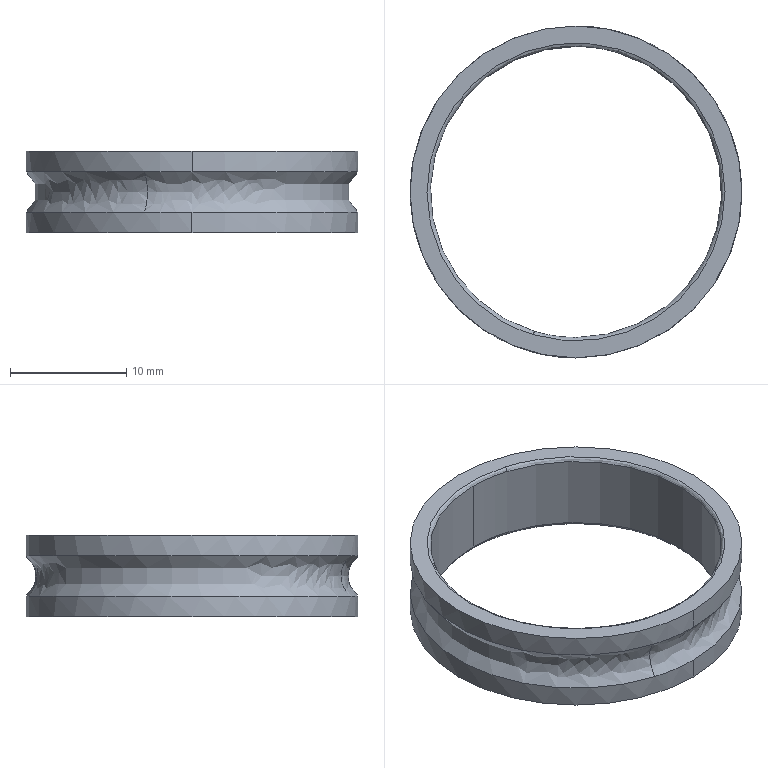Part | SolidWorks | features BaseBody 1 | 1 solid | 14 faces | box 28.5 x 28.5 x 7 mm | volume 836.369 mm3 | spline 6 | cylinder 6 | plane 2 | commonest cylinder face diameters 28.5 x4 25 x2
STEP:
#1=CARTESIAN_POINT('',(513.262,2.017,252.244));
#2=VERTEX_POINT('',#1);
#3=CARTESIAN_POINT('',(516.849,1.491,252.244));
#4=VERTEX_POINT('',#3);
#5=CARTESIAN_POINT('',(513.262,-10.483,252.244));
#6=DIRECTION('',(-0.000000004,0.00000001,-1.));
#7=DIRECTION('',(0.,-1.,-0.00000001));
#8=AXIS2_PLACEMENT_3D('',#5,#6,#7);
#9=CIRCLE('',#8,12.5);
#10=EDGE_CURVE('',#2,#4,#9,.T.);
#11=ORIENTED_EDGE('',*,*,#10,.T.);
#12=CARTESIAN_POINT('',(516.935,1.778,252.544));
#13=VERTEX_POINT('',#12);
#14=CARTESIAN_POINT('',(516.935,1.778,252.244));
#15=DIRECTION('',(-0.9579,0.287,0.000000007));
#16=DIRECTION('',(0.287,0.9579,0.000000008));
#17=AXIS2_PLACEMENT_3D('',#14,#15,#16);
#18=CIRCLE('',#17,0.3);
#19=EDGE_CURVE('',#4,#13,#18,.T.);
#20=ORIENTED_EDGE('',*,*,#19,.T.);
#21=CARTESIAN_POINT('',(509.588,-22.745,252.544));
#22=VERTEX_POINT('',#21);
#23=CARTESIAN_POINT('',(516.935,1.778,252.544));
#24=CARTESIAN_POINT('',(492.413,9.126,252.544));
#25=CARTESIAN_POINT('',(485.065,-15.397,252.544));
#26=CARTESIAN_POINT('',(509.588,-22.745,252.544));
#27=(BOUNDED_CURVE()B_SPLINE_CURVE(3,(#23,#24,#25,#26),.UNSPECIFIED.,.F.,.T.)B_SPLINE_CURVE_WITH_KNOTS((4,4),(0.,1.),.UNSPECIFIED.)CURVE()GEOMETRIC_REPRESENTATION_ITEM()RATIONAL_B_SPLINE_CURVE((1.,0.3333,0.3333,1.))REPRESENTATION_ITEM(''));
#28=EDGE_CURVE('',#13,#22,#27,.T.);
#29=ORIENTED_EDGE('',*,*,#28,.T.);
#30=CARTESIAN_POINT('',(509.674,-22.457,252.244));
#31=VERTEX_POINT('',#30);
#32=CARTESIAN_POINT('',(509.588,-22.745,252.244));
#33=DIRECTION('',(0.9579,-0.287,-0.000000007));
#34=DIRECTION('',(-0.287,-0.9579,-0.000000008));
#35=AXIS2_PLACEMENT_3D('',#32,#33,#34);
#36=CIRCLE('',#35,0.3);
#37=EDGE_CURVE('',#31,#22,#36,.T.);
#38=ORIENTED_EDGE('',*,*,#37,.F.);
#39=CARTESIAN_POINT('',(513.262,-10.483,252.244));
#40=DIRECTION('',(-0.000000004,0.00000001,-1.));
#41=DIRECTION('',(0.,-1.,-0.00000001));
#42=AXIS2_PLACEMENT_3D('',#39,#40,#41);
#43=CIRCLE('',#42,12.5);
#44=EDGE_CURVE('',#31,#2,#43,.T.);
#45=ORIENTED_EDGE('',*,*,#44,.T.);
#46=EDGE_LOOP('',(#11,#20,#29,#38,#45));
#47=FACE_OUTER_BOUND('',#46,.T.);
#48=CARTESIAN_POINT('',(516.849,1.491,252.244));
#49=CARTESIAN_POINT('',(492.901,8.666,252.244));
#50=CARTESIAN_POINT('',(485.726,-15.282,252.244));
#51=CARTESIAN_POINT('',(509.674,-22.457,252.244));
#52=CARTESIAN_POINT('',(516.849,1.491,252.42));
#53=CARTESIAN_POINT('',(492.901,8.666,252.42));
#54=CARTESIAN_POINT('',(485.726,-15.282,252.42));
#55=CARTESIAN_POINT('',(509.674,-22.457,252.42));
#56=CARTESIAN_POINT('',(516.885,1.61,252.544));
#57=CARTESIAN_POINT('',(492.699,8.857,252.544));
#58=CARTESIAN_POINT('',(485.452,-15.33,252.544));
#59=CARTESIAN_POINT('',(509.638,-22.576,252.544));
#60=CARTESIAN_POINT('',(516.935,1.778,252.544));
#61=CARTESIAN_POINT('',(492.413,9.126,252.544));
#62=CARTESIAN_POINT('',(485.065,-15.397,252.544));
#63=CARTESIAN_POINT('',(509.588,-22.745,252.544));
#64=(BOUNDED_SURFACE()B_SPLINE_SURFACE(3,3,((#48,#49,#50,#51),(#52,#53,#54,#55),(#56,#57,#58,#59),(#60,#61,#62,#63)),.UNSPECIFIED.,.F.,.F.,.T.)B_SPLINE_SURFACE_WITH_KNOTS((4,4),(4,4),(0.,1.),(0.,1.),.UNSPECIFIED.)GEOMETRIC_REPRESENTATION_ITEM()RATIONAL_B_SPLINE_SURFACE(((1.,0.3333,0.3333,1.),(0.8047,0.2682,0.2682,0.8047),(0.8047,0.2682,0.2682,0.8047),(1.,0.3333,0.3333,1.)))REPRESENTATION_ITEM('')SURFACE());
#65=ADVANCED_FACE('',(#47),#64,.T.);
#66=CARTESIAN_POINT('',(509.588,-22.745,245.544));
#67=VERTEX_POINT('',#66);
#68=CARTESIAN_POINT('',(516.935,1.778,245.544));
#69=VERTEX_POINT('',#68);
#70=CARTESIAN_POINT('',(509.588,-22.745,245.544));
#71=CARTESIAN_POINT('',(485.065,-15.397,245.544));
#72=CARTESIAN_POINT('',(492.413,9.126,245.544));
#73=CARTESIAN_POINT('',(516.935,1.778,245.544));
#74=(BOUNDED_CURVE()B_SPLINE_CURVE(3,(#70,#71,#72,#73),.UNSPECIFIED.,.F.,.T.)B_SPLINE_CURVE_WITH_KNOTS((4,4),(0.,1.),.UNSPECIFIED.)CURVE()GEOMETRIC_REPRESENTATION_ITEM()RATIONAL_B_SPLINE_CURVE((1.,0.3333,0.3333,1.))REPRESENTATION_ITEM(''));
#75=EDGE_CURVE('',#67,#69,#74,.T.);
#76=ORIENTED_EDGE('',*,*,#75,.T.);
#77=CARTESIAN_POINT('',(516.849,1.491,245.844));
#78=VERTEX_POINT('',#77);
#79=CARTESIAN_POINT('',(516.935,1.778,245.844));
#80=DIRECTION('',(-0.9579,0.287,0.000000007));
#81=DIRECTION('',(0.287,0.9579,0.000000008));
#82=AXIS2_PLACEMENT_3D('',#79,#80,#81);
#83=CIRCLE('',#82,0.3);
#84=EDGE_CURVE('',#69,#78,#83,.T.);
#85=ORIENTED_EDGE('',*,*,#84,.T.);
#86=CARTESIAN_POINT('',(513.262,2.017,245.844));
#87=VERTEX_POINT('',#86);
#88=CARTESIAN_POINT('',(513.262,-10.483,245.844));
#89=DIRECTION('',(0.000000004,-0.00000001,1.));
#90=DIRECTION('',(0.,-1.,-0.00000001));
#91=AXIS2_PLACEMENT_3D('',#88,#89,#90);
#92=CIRCLE('',#91,12.5);
#93=EDGE_CURVE('',#78,#87,#92,.T.);
#94=ORIENTED_EDGE('',*,*,#93,.T.);
#95=CARTESIAN_POINT('',(509.674,-22.457,245.844));
#96=VERTEX_POINT('',#95);
#97=CARTESIAN_POINT('',(513.262,-10.483,245.844));
#98=DIRECTION('',(0.000000004,-0.00000001,1.));
#99=DIRECTION('',(0.,-1.,-0.00000001));
#100=AXIS2_PLACEMENT_3D('',#97,#98,#99);
#101=CIRCLE('',#100,12.5);
#102=EDGE_CURVE('',#87,#96,#101,.T.);
#103=ORIENTED_EDGE('',*,*,#102,.T.);
#104=CARTESIAN_POINT('',(509.588,-22.745,245.844));
#105=DIRECTION('',(0.9579,-0.287,-0.000000007));
#106=DIRECTION('',(-0.287,-0.9579,-0.000000008));
#107=AXIS2_PLACEMENT_3D('',#104,#105,#106);
#108=CIRCLE('',#107,0.3);
#109=EDGE_CURVE('',#67,#96,#108,.T.);
#110=ORIENTED_EDGE('',*,*,#109,.F.);
#111=EDGE_LOOP('',(#76,#85,#94,#103,#110));
#112=FACE_OUTER_BOUND('',#111,.T.);
#113=CARTESIAN_POINT('',(516.935,1.778,245.544));
#114=CARTESIAN_POINT('',(492.413,9.126,245.544));
#115=CARTESIAN_POINT('',(485.065,-15.397,245.544));
#116=CARTESIAN_POINT('',(509.588,-22.745,245.544));
#117=CARTESIAN_POINT('',(516.885,1.61,245.544));
#118=CARTESIAN_POINT('',(492.699,8.857,245.544));
#119=CARTESIAN_POINT('',(485.452,-15.33,245.544));
#120=CARTESIAN_POINT('',(509.638,-22.576,245.544));
#121=CARTESIAN_POINT('',(516.849,1.491,245.669));
#122=CARTESIAN_POINT('',(492.901,8.666,245.669));
#123=CARTESIAN_POINT('',(485.726,-15.282,245.669));
#124=CARTESIAN_POINT('',(509.674,-22.457,245.669));
#125=CARTESIAN_POINT('',(516.849,1.491,245.844));
#126=CARTESIAN_POINT('',(492.901,8.666,245.844));
#127=CARTESIAN_POINT('',(485.726,-15.282,245.844));
#128=CARTESIAN_POINT('',(509.674,-22.457,245.844));
#129=(BOUNDED_SURFACE()B_SPLINE_SURFACE(3,3,((#113,#114,#115,#116),(#117,#118,#119,#120),(#121,#122,#123,#124),(#125,#126,#127,#128)),.UNSPECIFIED.,.F.,.F.,.T.)B_SPLINE_SURFACE_WITH_KNOTS((4,4),(4,4),(0.,1.),(0.,1.),.UNSPECIFIED.)GEOMETRIC_REPRESENTATION_ITEM()RATIONAL_B_SPLINE_SURFACE(((1.,0.3333,0.3333,1.),(0.8047,0.2682,0.2682,0.8047),(0.8047,0.2682,0.2682,0.8047),(1.,0.3333,0.3333,1.)))REPRESENTATION_ITEM('')SURFACE());
#130=ADVANCED_FACE('',(#112),#129,.T.);
#131=CARTESIAN_POINT('',(517.352,3.167,247.321));
#132=VERTEX_POINT('',#131);
#133=CARTESIAN_POINT('',(513.262,-24.733,247.321));
#134=VERTEX_POINT('',#133);
#135=CARTESIAN_POINT('',(513.262,-10.483,247.321));
#136=DIRECTION('',(-0.000000004,0.00000001,-1.));
#137=DIRECTION('',(0.,-1.,-0.00000001));
#138=AXIS2_PLACEMENT_3D('',#135,#136,#137);
#139=CIRCLE('',#138,14.25);
#140=EDGE_CURVE('',#132,#134,#139,.T.);
#141=ORIENTED_EDGE('',*,*,#140,.F.);
#142=CARTESIAN_POINT('',(517.352,3.167,250.768));
#143=VERTEX_POINT('',#142);
#144=CARTESIAN_POINT('',(517.696,4.317,249.044));
#145=DIRECTION('',(-0.9579,0.287,0.000000007));
#146=DIRECTION('',(0.287,0.9579,0.000000008));
#147=AXIS2_PLACEMENT_3D('',#144,#145,#146);
#148=CIRCLE('',#147,2.1);
#149=EDGE_CURVE('',#132,#143,#148,.T.);
#150=ORIENTED_EDGE('',*,*,#149,.T.);
#151=CARTESIAN_POINT('',(513.262,-24.733,250.768));
#152=VERTEX_POINT('',#151);
#153=CARTESIAN_POINT('',(513.262,-10.483,250.768));
#154=DIRECTION('',(0.000000004,-0.00000001,1.));
#155=DIRECTION('',(0.,-1.,-0.00000001));
#156=AXIS2_PLACEMENT_3D('',#153,#154,#155);
#157=CIRCLE('',#156,14.25);
#158=EDGE_CURVE('',#152,#143,#157,.T.);
#159=ORIENTED_EDGE('',*,*,#158,.F.);
#160=CARTESIAN_POINT('',(509.171,-24.134,250.768));
#161=VERTEX_POINT('',#160);
#162=CARTESIAN_POINT('',(513.262,-10.483,250.768));
#163=DIRECTION('',(0.000000004,-0.00000001,1.));
#164=DIRECTION('',(0.,-1.,-0.00000001));
#165=AXIS2_PLACEMENT_3D('',#162,#163,#164);
#166=CIRCLE('',#165,14.25);
#167=EDGE_CURVE('',#161,#152,#166,.T.);
#168=ORIENTED_EDGE('',*,*,#167,.F.);
#169=CARTESIAN_POINT('',(509.171,-24.134,247.321));
#170=VERTEX_POINT('',#169);
#171=CARTESIAN_POINT('',(508.827,-25.283,249.044));
#172=DIRECTION('',(0.9579,-0.287,-0.000000007));
#173=DIRECTION('',(-0.287,-0.9579,-0.000000008));
#174=AXIS2_PLACEMENT_3D('',#171,#172,#173);
#175=CIRCLE('',#174,2.1);
#176=EDGE_CURVE('',#170,#161,#175,.T.);
#177=ORIENTED_EDGE('',*,*,#176,.F.);
#178=CARTESIAN_POINT('',(513.262,-10.483,247.321));
#179=DIRECTION('',(-0.000000004,0.00000001,-1.));
#180=DIRECTION('',(0.,-1.,-0.00000001));
#181=AXIS2_PLACEMENT_3D('',#178,#179,#180);
#182=CIRCLE('',#181,14.25);
#183=EDGE_CURVE('',#134,#170,#182,.T.);
#184=ORIENTED_EDGE('',*,*,#183,.F.);
#185=EDGE_LOOP('',(#141,#150,#159,#168,#177,#184));
#186=FACE_OUTER_BOUND('',#185,.T.);
#187=CARTESIAN_POINT('',(509.171,-24.134,247.321));
#188=CARTESIAN_POINT('',(536.472,-32.314,247.321));
#189=CARTESIAN_POINT('',(544.652,-5.013,247.321));
#190=CARTESIAN_POINT('',(517.352,3.167,247.321));
#191=CARTESIAN_POINT('',(509.55,-22.869,248.24));
#192=CARTESIAN_POINT('',(534.322,-30.292,248.24));
#193=CARTESIAN_POINT('',(541.745,-5.52,248.24));
#194=CARTESIAN_POINT('',(516.973,1.903,248.24));
#195=CARTESIAN_POINT('',(509.55,-22.869,249.848));
#196=CARTESIAN_POINT('',(534.322,-30.292,249.848));
#197=CARTESIAN_POINT('',(541.745,-5.52,249.848));
#198=CARTESIAN_POINT('',(516.973,1.903,249.848));
#199=CARTESIAN_POINT('',(509.171,-24.134,250.768));
#200=CARTESIAN_POINT('',(536.472,-32.314,250.768));
#201=CARTESIAN_POINT('',(544.652,-5.013,250.768));
#202=CARTESIAN_POINT('',(517.352,3.167,250.768));
#203=(BOUNDED_SURFACE()B_SPLINE_SURFACE(3,3,((#187,#188,#189,#190),(#191,#192,#193,#194),(#195,#196,#197,#198),(#199,#200,#201,#202)),.UNSPECIFIED.,.F.,.F.,.T.)B_SPLINE_SURFACE_WITH_KNOTS((4,4),(4,4),(0.,1.),(0.,1.),.UNSPECIFIED.)GEOMETRIC_REPRESENTATION_ITEM()RATIONAL_B_SPLINE_SURFACE(((1.,0.3333,0.3333,1.),(0.7143,0.2381,0.2381,0.7143),(0.7143,0.2381,0.2381,0.7143),(1.,0.3333,0.3333,1.)))REPRESENTATION_ITEM('')SURFACE());
#204=ADVANCED_FACE('',(#186),#203,.F.);
#205=ORIENTED_EDGE('',*,*,#102,.F.);
#206=CARTESIAN_POINT('',(513.262,2.017,249.044));
#207=DIRECTION('',(0.000000004,-0.00000001,1.));
#208=VECTOR('',#207,1000.);
#209=LINE('',#206,#208);
#210=EDGE_CURVE('',#87,#2,#209,.T.);
#211=ORIENTED_EDGE('',*,*,#210,.T.);
#212=ORIENTED_EDGE('',*,*,#44,.F.);
#213=CARTESIAN_POINT('',(513.262,-22.983,252.244));
#214=VERTEX_POINT('',#213);
#215=CARTESIAN_POINT('',(513.262,-10.483,252.244));
#216=DIRECTION('',(-0.000000004,0.00000001,-1.));
#217=DIRECTION('',(0.,-1.,-0.00000001));
#218=AXIS2_PLACEMENT_3D('',#215,#216,#217);
#219=CIRCLE('',#218,12.5);
#220=EDGE_CURVE('',#214,#31,#219,.T.);
#221=ORIENTED_EDGE('',*,*,#220,.F.);
#222=CARTESIAN_POINT('',(513.262,-22.983,245.844));
#223=VERTEX_POINT('',#222);
#224=CARTESIAN_POINT('',(513.262,-22.983,249.044));
#225=DIRECTION('',(0.000000004,-0.00000001,1.));
#226=VECTOR('',#225,1000.);
#227=LINE('',#224,#226);
#228=EDGE_CURVE('',#223,#214,#227,.T.);
#229=ORIENTED_EDGE('',*,*,#228,.F.);
#230=CARTESIAN_POINT('',(513.262,-10.483,245.844));
#231=DIRECTION('',(0.000000004,-0.00000001,1.));
#232=DIRECTION('',(0.,-1.,-0.00000001));
#233=AXIS2_PLACEMENT_3D('',#230,#231,#232);
#234=CIRCLE('',#233,12.5);
#235=EDGE_CURVE('',#96,#223,#234,.T.);
#236=ORIENTED_EDGE('',*,*,#235,.F.);
#237=EDGE_LOOP('',(#205,#211,#212,#221,#229,#236));
#238=FACE_OUTER_BOUND('',#237,.T.);
#239=CARTESIAN_POINT('',(513.262,-10.483,249.044));
#240=DIRECTION('',(0.000000004,-0.00000001,1.));
#241=DIRECTION('',(0.,-1.,-0.00000001));
#242=AXIS2_PLACEMENT_3D('',#239,#240,#241);
#243=CYLINDRICAL_SURFACE('',#242,12.5);
#244=ADVANCED_FACE('',(#238),#243,.F.);
#245=ORIENTED_EDGE('',*,*,#158,.T.);
#246=CARTESIAN_POINT('',(513.262,3.767,250.768));
#247=VERTEX_POINT('',#246);
#248=CARTESIAN_POINT('',(513.262,-10.483,250.768));
#249=DIRECTION('',(0.000000004,-0.00000001,1.));
#250=DIRECTION('',(0.,-1.,-0.00000001));
#251=AXIS2_PLACEMENT_3D('',#248,#249,#250);
#252=CIRCLE('',#251,14.25);
#253=EDGE_CURVE('',#143,#247,#252,.T.);
#254=ORIENTED_EDGE('',*,*,#253,.T.);
#255=CARTESIAN_POINT('',(513.262,3.767,252.544));
#256=VERTEX_POINT('',#255);
#257=CARTESIAN_POINT('',(513.262,3.767,251.656));
#258=DIRECTION('',(0.000000004,-0.00000001,1.));
#259=VECTOR('',#258,1000.);
#260=LINE('',#257,#259);
#261=EDGE_CURVE('',#247,#256,#260,.T.);
#262=ORIENTED_EDGE('',*,*,#261,.T.);
#263=CARTESIAN_POINT('',(513.262,-24.733,252.544));
#264=VERTEX_POINT('',#263);
#265=CARTESIAN_POINT('',(513.262,-10.483,252.544));
#266=DIRECTION('',(0.000000004,-0.00000001,1.));
#267=DIRECTION('',(0.,-1.,-0.00000001));
#268=AXIS2_PLACEMENT_3D('',#265,#266,#267);
#269=CIRCLE('',#268,14.25);
#270=EDGE_CURVE('',#264,#256,#269,.T.);
#271=ORIENTED_EDGE('',*,*,#270,.F.);
#272=CARTESIAN_POINT('',(513.262,-24.733,251.656));
#273=DIRECTION('',(0.000000004,-0.00000001,1.));
#274=VECTOR('',#273,1000.);
#275=LINE('',#272,#274);
#276=EDGE_CURVE('',#152,#264,#275,.T.);
#277=ORIENTED_EDGE('',*,*,#276,.F.);
#278=EDGE_LOOP('',(#245,#254,#262,#271,#277));
#279=FACE_OUTER_BOUND('',#278,.T.);
#280=CARTESIAN_POINT('',(513.262,-10.483,251.656));
#281=DIRECTION('',(0.000000004,-0.00000001,1.));
#282=DIRECTION('',(0.,-1.,-0.00000001));
#283=AXIS2_PLACEMENT_3D('',#280,#281,#282);
#284=CYLINDRICAL_SURFACE('',#283,14.25);
#285=ADVANCED_FACE('',(#279),#284,.T.);
#286=CARTESIAN_POINT('',(513.262,3.767,245.544));
#287=VERTEX_POINT('',#286);
#288=CARTESIAN_POINT('',(513.262,-24.733,245.544));
#289=VERTEX_POINT('',#288);
#290=CARTESIAN_POINT('',(513.262,-10.483,245.544));
#291=DIRECTION('',(-0.000000004,0.00000001,-1.));
#292=DIRECTION('',(0.,-1.,-0.00000001));
#293=AXIS2_PLACEMENT_3D('',#290,#291,#292);
#294=CIRCLE('',#293,14.25);
#295=EDGE_CURVE('',#287,#289,#294,.T.);
#296=ORIENTED_EDGE('',*,*,#295,.F.);
#297=CARTESIAN_POINT('',(513.262,3.767,247.321));
#298=VERTEX_POINT('',#297);
#299=CARTESIAN_POINT('',(513.262,3.767,246.433));
#300=DIRECTION('',(0.000000004,-0.00000001,1.));
#301=VECTOR('',#300,1000.);
#302=LINE('',#299,#301);
#303=EDGE_CURVE('',#287,#298,#302,.T.);
#304=ORIENTED_EDGE('',*,*,#303,.T.);
#305=CARTESIAN_POINT('',(513.262,-10.483,247.321));
#306=DIRECTION('',(-0.000000004,0.00000001,-1.));
#307=DIRECTION('',(0.,-1.,-0.00000001));
#308=AXIS2_PLACEMENT_3D('',#305,#306,#307);
#309=CIRCLE('',#308,14.25);
#310=EDGE_CURVE('',#298,#132,#309,.T.);
#311=ORIENTED_EDGE('',*,*,#310,.T.);
#312=ORIENTED_EDGE('',*,*,#140,.T.);
#313=CARTESIAN_POINT('',(513.262,-24.733,246.433));
#314=DIRECTION('',(0.000000004,-0.00000001,1.));
#315=VECTOR('',#314,1000.);
#316=LINE('',#313,#315);
#317=EDGE_CURVE('',#289,#134,#316,.T.);
#318=ORIENTED_EDGE('',*,*,#317,.F.);
#319=EDGE_LOOP('',(#296,#304,#311,#312,#318));
#320=FACE_OUTER_BOUND('',#319,.T.);
#321=CARTESIAN_POINT('',(513.262,-10.483,246.433));
#322=DIRECTION('',(0.000000004,-0.00000001,1.));
#323=DIRECTION('',(0.,-1.,-0.00000001));
#324=AXIS2_PLACEMENT_3D('',#321,#322,#323);
#325=CYLINDRICAL_SURFACE('',#324,14.25);
#326=ADVANCED_FACE('',(#320),#325,.T.);
#327=ORIENTED_EDGE('',*,*,#210,.F.);
#328=ORIENTED_EDGE('',*,*,#93,.F.);
#329=CARTESIAN_POINT('',(513.262,-10.483,245.844));
#330=DIRECTION('',(0.000000004,-0.00000001,1.));
#331=DIRECTION('',(0.,-1.,-0.00000001));
#332=AXIS2_PLACEMENT_3D('',#329,#330,#331);
#333=CIRCLE('',#332,12.5);
#334=EDGE_CURVE('',#223,#78,#333,.T.);
#335=ORIENTED_EDGE('',*,*,#334,.F.);
#336=ORIENTED_EDGE('',*,*,#228,.T.);
#337=CARTESIAN_POINT('',(513.262,-10.483,252.244));
#338=DIRECTION('',(-0.000000004,0.00000001,-1.));
#339=DIRECTION('',(0.,-1.,-0.00000001));
#340=AXIS2_PLACEMENT_3D('',#337,#338,#339);
#341=CIRCLE('',#340,12.5);
#342=EDGE_CURVE('',#4,#214,#341,.T.);
#343=ORIENTED_EDGE('',*,*,#342,.F.);
#344=ORIENTED_EDGE('',*,*,#10,.F.);
#345=EDGE_LOOP('',(#327,#328,#335,#336,#343,#344));
#346=FACE_OUTER_BOUND('',#345,.T.);
#347=CARTESIAN_POINT('',(513.262,-10.483,249.044));
#348=DIRECTION('',(0.000000004,-0.00000001,1.));
#349=DIRECTION('',(0.,-1.,-0.00000001));
#350=AXIS2_PLACEMENT_3D('',#347,#348,#349);
#351=CYLINDRICAL_SURFACE('',#350,12.5);
#352=ADVANCED_FACE('',(#346),#351,.F.);
#353=ORIENTED_EDGE('',*,*,#19,.F.);
#354=ORIENTED_EDGE('',*,*,#342,.T.);
#355=ORIENTED_EDGE('',*,*,#220,.T.);
#356=ORIENTED_EDGE('',*,*,#37,.T.);
#357=CARTESIAN_POINT('',(509.588,-22.745,252.544));
#358=CARTESIAN_POINT('',(534.111,-30.093,252.544));
#359=CARTESIAN_POINT('',(541.458,-5.57,252.544));
#360=CARTESIAN_POINT('',(516.935,1.778,252.544));
#361=(BOUNDED_CURVE()B_SPLINE_CURVE(3,(#357,#358,#359,#360),.UNSPECIFIED.,.F.,.T.)B_SPLINE_CURVE_WITH_KNOTS((4,4),(0.,1.),.UNSPECIFIED.)CURVE()GEOMETRIC_REPRESENTATION_ITEM()RATIONAL_B_SPLINE_CURVE((1.,0.3333,0.3333,1.))REPRESENTATION_ITEM(''));
#362=EDGE_CURVE('',#22,#13,#361,.T.);
#363=ORIENTED_EDGE('',*,*,#362,.T.);
#364=EDGE_LOOP('',(#353,#354,#355,#356,#363));
#365=FACE_OUTER_BOUND('',#364,.T.);
#366=CARTESIAN_POINT('',(509.674,-22.457,252.244));
#367=CARTESIAN_POINT('',(533.622,-29.633,252.244));
#368=CARTESIAN_POINT('',(540.797,-5.685,252.244));
#369=CARTESIAN_POINT('',(516.849,1.491,252.244));
#370=CARTESIAN_POINT('',(509.674,-22.457,252.42));
#371=CARTESIAN_POINT('',(533.622,-29.633,252.42));
#372=CARTESIAN_POINT('',(540.797,-5.685,252.42));
#373=CARTESIAN_POINT('',(516.849,1.491,252.42));
#374=CARTESIAN_POINT('',(509.638,-22.576,252.544));
#375=CARTESIAN_POINT('',(533.824,-29.823,252.544));
#376=CARTESIAN_POINT('',(541.071,-5.637,252.544));
#377=CARTESIAN_POINT('',(516.885,1.61,252.544));
#378=CARTESIAN_POINT('',(509.588,-22.745,252.544));
#379=CARTESIAN_POINT('',(534.111,-30.093,252.544));
#380=CARTESIAN_POINT('',(541.458,-5.57,252.544));
#381=CARTESIAN_POINT('',(516.935,1.778,252.544));
#382=(BOUNDED_SURFACE()B_SPLINE_SURFACE(3,3,((#366,#367,#368,#369),(#370,#371,#372,#373),(#374,#375,#376,#377),(#378,#379,#380,#381)),.UNSPECIFIED.,.F.,.F.,.F.)B_SPLINE_SURFACE_WITH_KNOTS((4,4),(4,4),(0.,1.),(0.,1.),.UNSPECIFIED.)GEOMETRIC_REPRESENTATION_ITEM()RATIONAL_B_SPLINE_SURFACE(((1.,0.3333,0.3333,1.),(0.8047,0.2682,0.2682,0.8047),(0.8047,0.2682,0.2682,0.8047),(1.,0.3333,0.3333,1.)))REPRESENTATION_ITEM('')SURFACE());
#383=ADVANCED_FACE('',(#365),#382,.T.);
#384=ORIENTED_EDGE('',*,*,#84,.F.);
#385=CARTESIAN_POINT('',(516.935,1.778,245.544));
#386=CARTESIAN_POINT('',(541.458,-5.57,245.544));
#387=CARTESIAN_POINT('',(534.111,-30.093,245.544));
#388=CARTESIAN_POINT('',(509.588,-22.745,245.544));
#389=(BOUNDED_CURVE()B_SPLINE_CURVE(3,(#385,#386,#387,#388),.UNSPECIFIED.,.F.,.T.)B_SPLINE_CURVE_WITH_KNOTS((4,4),(0.,1.),.UNSPECIFIED.)CURVE()GEOMETRIC_REPRESENTATION_ITEM()RATIONAL_B_SPLINE_CURVE((1.,0.3333,0.3333,1.))REPRESENTATION_ITEM(''));
#390=EDGE_CURVE('',#69,#67,#389,.T.);
#391=ORIENTED_EDGE('',*,*,#390,.T.);
#392=ORIENTED_EDGE('',*,*,#109,.T.);
#393=ORIENTED_EDGE('',*,*,#235,.T.);
#394=ORIENTED_EDGE('',*,*,#334,.T.);
#395=EDGE_LOOP('',(#384,#391,#392,#393,#394));
#396=FACE_OUTER_BOUND('',#395,.T.);
#397=CARTESIAN_POINT('',(509.588,-22.745,245.544));
#398=CARTESIAN_POINT('',(534.111,-30.093,245.544));
#399=CARTESIAN_POINT('',(541.458,-5.57,245.544));
#400=CARTESIAN_POINT('',(516.935,1.778,245.544));
#401=CARTESIAN_POINT('',(509.638,-22.576,245.544));
#402=CARTESIAN_POINT('',(533.824,-29.823,245.544));
#403=CARTESIAN_POINT('',(541.071,-5.637,245.544));
#404=CARTESIAN_POINT('',(516.885,1.61,245.544));
#405=CARTESIAN_POINT('',(509.674,-22.457,245.669));
#406=CARTESIAN_POINT('',(533.622,-29.633,245.669));
#407=CARTESIAN_POINT('',(540.797,-5.685,245.669));
#408=CARTESIAN_POINT('',(516.849,1.491,245.669));
#409=CARTESIAN_POINT('',(509.674,-22.457,245.844));
#410=CARTESIAN_POINT('',(533.622,-29.633,245.844));
#411=CARTESIAN_POINT('',(540.797,-5.685,245.844));
#412=CARTESIAN_POINT('',(516.849,1.491,245.844));
#413=(BOUNDED_SURFACE()B_SPLINE_SURFACE(3,3,((#397,#398,#399,#400),(#401,#402,#403,#404),(#405,#406,#407,#408),(#409,#410,#411,#412)),.UNSPECIFIED.,.F.,.F.,.T.)B_SPLINE_SURFACE_WITH_KNOTS((4,4),(4,4),(0.,1.),(0.,1.),.UNSPECIFIED.)GEOMETRIC_REPRESENTATION_ITEM()RATIONAL_B_SPLINE_SURFACE(((1.,0.3333,0.3333,1.),(0.8047,0.2682,0.2682,0.8047),(0.8047,0.2682,0.2682,0.8047),(1.,0.3333,0.3333,1.)))REPRESENTATION_ITEM('')SURFACE());
#414=ADVANCED_FACE('',(#396),#413,.T.);
#415=ORIENTED_EDGE('',*,*,#28,.F.);
#416=ORIENTED_EDGE('',*,*,#362,.F.);
#417=EDGE_LOOP('',(#415,#416));
#418=FACE_BOUND('',#417,.T.);
#419=ORIENTED_EDGE('',*,*,#270,.T.);
#420=CARTESIAN_POINT('',(513.262,-10.483,252.544));
#421=DIRECTION('',(0.000000004,-0.00000001,1.));
#422=DIRECTION('',(0.,-1.,-0.00000001));
#423=AXIS2_PLACEMENT_3D('',#420,#421,#422);
#424=CIRCLE('',#423,14.25);
#425=EDGE_CURVE('',#256,#264,#424,.T.);
#426=ORIENTED_EDGE('',*,*,#425,.T.);
#427=EDGE_LOOP('',(#419,#426));
#428=FACE_OUTER_BOUND('',#427,.T.);
#429=CARTESIAN_POINT('',(509.38,-23.439,252.544));
#430=DIRECTION('',(0.000000004,-0.00000001,1.));
#431=DIRECTION('',(0.,-1.,-0.00000001));
#432=AXIS2_PLACEMENT_3D('',#429,#430,#431);
#433=PLANE('',#432);
#434=ADVANCED_FACE('',(#418,#428),#433,.T.);
#435=CARTESIAN_POINT('',(513.262,-10.483,245.544));
#436=DIRECTION('',(-0.000000004,0.00000001,-1.));
#437=DIRECTION('',(0.,-1.,-0.00000001));
#438=AXIS2_PLACEMENT_3D('',#435,#436,#437);
#439=CIRCLE('',#438,14.25);
#440=EDGE_CURVE('',#289,#287,#439,.T.);
#441=ORIENTED_EDGE('',*,*,#440,.T.);
#442=ORIENTED_EDGE('',*,*,#295,.T.);
#443=EDGE_LOOP('',(#441,#442));
#444=FACE_OUTER_BOUND('',#443,.T.);
#445=ORIENTED_EDGE('',*,*,#75,.F.);
#446=ORIENTED_EDGE('',*,*,#390,.F.);
#447=EDGE_LOOP('',(#445,#446));
#448=FACE_BOUND('',#447,.T.);
#449=CARTESIAN_POINT('',(509.38,-23.439,245.544));
#450=DIRECTION('',(-0.000000004,0.00000001,-1.));
#451=DIRECTION('',(0.,1.,0.00000001));
#452=AXIS2_PLACEMENT_3D('',#449,#450,#451);
#453=PLANE('',#452);
#454=ADVANCED_FACE('',(#444,#448),#453,.T.);
#455=ORIENTED_EDGE('',*,*,#261,.F.);
#456=CARTESIAN_POINT('',(513.262,-10.483,250.768));
#457=DIRECTION('',(0.000000004,-0.00000001,1.));
#458=DIRECTION('',(0.,-1.,-0.00000001));
#459=AXIS2_PLACEMENT_3D('',#456,#457,#458);
#460=CIRCLE('',#459,14.25);
#461=EDGE_CURVE('',#247,#161,#460,.T.);
#462=ORIENTED_EDGE('',*,*,#461,.T.);
#463=ORIENTED_EDGE('',*,*,#167,.T.);
#464=ORIENTED_EDGE('',*,*,#276,.T.);
#465=ORIENTED_EDGE('',*,*,#425,.F.);
#466=EDGE_LOOP('',(#455,#462,#463,#464,#465));
#467=FACE_OUTER_BOUND('',#466,.T.);
#468=CARTESIAN_POINT('',(513.262,-10.483,251.656));
#469=DIRECTION('',(0.000000004,-0.00000001,1.));
#470=DIRECTION('',(0.,-1.,-0.00000001));
#471=AXIS2_PLACEMENT_3D('',#468,#469,#470);
#472=CYLINDRICAL_SURFACE('',#471,14.25);
#473=ADVANCED_FACE('',(#467),#472,.T.);
#474=ORIENTED_EDGE('',*,*,#303,.F.);
#475=ORIENTED_EDGE('',*,*,#440,.F.);
#476=ORIENTED_EDGE('',*,*,#317,.T.);
#477=ORIENTED_EDGE('',*,*,#183,.T.);
#478=CARTESIAN_POINT('',(513.262,-10.483,247.321));
#479=DIRECTION('',(-0.000000004,0.00000001,-1.));
#480=DIRECTION('',(0.,-1.,-0.00000001));
#481=AXIS2_PLACEMENT_3D('',#478,#479,#480);
#482=CIRCLE('',#481,14.25);
#483=EDGE_CURVE('',#170,#298,#482,.T.);
#484=ORIENTED_EDGE('',*,*,#483,.T.);
#485=EDGE_LOOP('',(#474,#475,#476,#477,#484));
#486=FACE_OUTER_BOUND('',#485,.T.);
#487=CARTESIAN_POINT('',(513.262,-10.483,246.433));
#488=DIRECTION('',(0.000000004,-0.00000001,1.));
#489=DIRECTION('',(0.,-1.,-0.00000001));
#490=AXIS2_PLACEMENT_3D('',#487,#488,#489);
#491=CYLINDRICAL_SURFACE('',#490,14.25);
#492=ADVANCED_FACE('',(#486),#491,.T.);
#493=ORIENTED_EDGE('',*,*,#149,.F.);
#494=ORIENTED_EDGE('',*,*,#310,.F.);
#495=ORIENTED_EDGE('',*,*,#483,.F.);
#496=ORIENTED_EDGE('',*,*,#176,.T.);
#497=ORIENTED_EDGE('',*,*,#461,.F.);
#498=ORIENTED_EDGE('',*,*,#253,.F.);
#499=EDGE_LOOP('',(#493,#494,#495,#496,#497,#498));
#500=FACE_OUTER_BOUND('',#499,.T.);
#501=CARTESIAN_POINT('',(517.352,3.167,247.321));
#502=CARTESIAN_POINT('',(490.051,11.347,247.321));
#503=CARTESIAN_POINT('',(481.871,-15.954,247.321));
#504=CARTESIAN_POINT('',(509.171,-24.134,247.321));
#505=CARTESIAN_POINT('',(516.973,1.903,248.24));
#506=CARTESIAN_POINT('',(492.201,9.325,248.24));
#507=CARTESIAN_POINT('',(484.778,-15.447,248.24));
#508=CARTESIAN_POINT('',(509.55,-22.869,248.24));
#509=CARTESIAN_POINT('',(516.973,1.903,249.848));
#510=CARTESIAN_POINT('',(492.201,9.325,249.848));
#511=CARTESIAN_POINT('',(484.778,-15.447,249.848));
#512=CARTESIAN_POINT('',(509.55,-22.869,249.848));
#513=CARTESIAN_POINT('',(517.352,3.167,250.768));
#514=CARTESIAN_POINT('',(490.051,11.347,250.768));
#515=CARTESIAN_POINT('',(481.871,-15.954,250.768));
#516=CARTESIAN_POINT('',(509.171,-24.134,250.768));
#517=(BOUNDED_SURFACE()B_SPLINE_SURFACE(3,3,((#501,#502,#503,#504),(#505,#506,#507,#508),(#509,#510,#511,#512),(#513,#514,#515,#516)),.UNSPECIFIED.,.F.,.F.,.F.)B_SPLINE_SURFACE_WITH_KNOTS((4,4),(4,4),(0.,1.),(0.,1.),.UNSPECIFIED.)GEOMETRIC_REPRESENTATION_ITEM()RATIONAL_B_SPLINE_SURFACE(((1.,0.3333,0.3333,1.),(0.7143,0.2381,0.2381,0.7143),(0.7143,0.2381,0.2381,0.7143),(1.,0.3333,0.3333,1.)))REPRESENTATION_ITEM('')SURFACE());
#518=ADVANCED_FACE('',(#500),#517,.F.);
#519=CLOSED_SHELL('',(#65,#130,#204,#244,#285,#326,#352,#383,#414,#434,#454,#473,#492,#518));
#520=MANIFOLD_SOLID_BREP('',#519);
#521=CARTESIAN_POINT('',(0.,0.,0.));
#522=DIRECTION('',(0.,0.,1.));
#523=DIRECTION('',(1.,0.,0.));
#524=AXIS2_PLACEMENT_3D('',#521,#522,#523);
#525=(LENGTH_UNIT()NAMED_UNIT(*)SI_UNIT(.MILLI.,.METRE.));
#526=UNCERTAINTY_MEASURE_WITH_UNIT(LENGTH_MEASURE(0.00001),#525,'','');
#527=(NAMED_UNIT(*)PLANE_ANGLE_UNIT()SI_UNIT($,.RADIAN.));
#528=(NAMED_UNIT(*)SI_UNIT($,.STERADIAN.)SOLID_ANGLE_UNIT());
#529=(GEOMETRIC_REPRESENTATION_CONTEXT(3)GLOBAL_UNCERTAINTY_ASSIGNED_CONTEXT((#526))GLOBAL_UNIT_ASSIGNED_CONTEXT((#525,#527,#528))REPRESENTATION_CONTEXT('',''));
#530=ADVANCED_BREP_SHAPE_REPRESENTATION('',(#520,#524),#529);